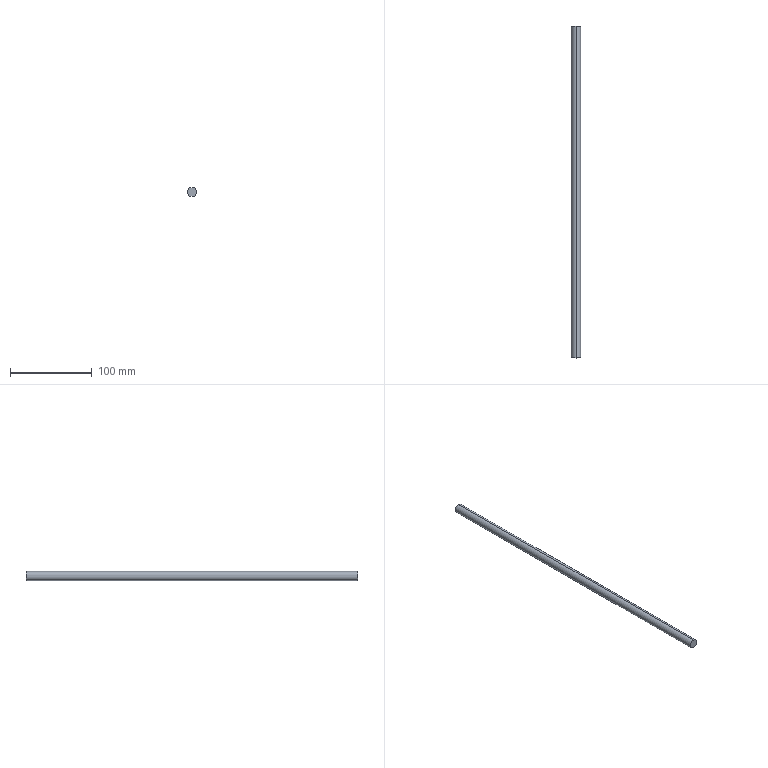Part | STEP file | 4-20.sldasm-Part-405 | 1 solid | 4 faces | box 11.11 x 405 x 11.11 mm | volume 39262 mm3 | cylinder 2 | plane 2 | commonest cylinder face diameters 11.11 x2
STEP:
#1=CARTESIAN_POINT('',(45.,-405.,179.555));
#2=VERTEX_POINT('',#1);
#3=CARTESIAN_POINT('',(45.,-405.,168.445));
#4=VERTEX_POINT('',#3);
#5=CARTESIAN_POINT('',(45.,-405.,174.));
#6=DIRECTION('',(0.,1.,0.));
#7=DIRECTION('',(0.,0.,1.));
#8=AXIS2_PLACEMENT_3D('',#5,#6,#7);
#9=CIRCLE('',#8,5.555);
#10=EDGE_CURVE('',#2,#4,#9,.T.);
#11=ORIENTED_EDGE('',*,*,#10,.T.);
#12=CARTESIAN_POINT('',(45.,0.,168.445));
#13=VERTEX_POINT('',#12);
#14=CARTESIAN_POINT('',(45.,-430.,168.445));
#15=DIRECTION('',(0.,1.,0.));
#16=VECTOR('',#15,1000.);
#17=LINE('',#14,#16);
#18=EDGE_CURVE('',#4,#13,#17,.T.);
#19=ORIENTED_EDGE('',*,*,#18,.T.);
#20=CARTESIAN_POINT('',(45.,0.,179.555));
#21=VERTEX_POINT('',#20);
#22=CARTESIAN_POINT('',(45.,0.,174.));
#23=DIRECTION('',(0.,-1.,0.));
#24=DIRECTION('',(0.,0.,-1.));
#25=AXIS2_PLACEMENT_3D('',#22,#23,#24);
#26=CIRCLE('',#25,5.555);
#27=EDGE_CURVE('',#13,#21,#26,.T.);
#28=ORIENTED_EDGE('',*,*,#27,.T.);
#29=CARTESIAN_POINT('',(45.,-430.,179.555));
#30=DIRECTION('',(0.,1.,0.));
#31=VECTOR('',#30,1000.);
#32=LINE('',#29,#31);
#33=EDGE_CURVE('',#2,#21,#32,.T.);
#34=ORIENTED_EDGE('',*,*,#33,.F.);
#35=EDGE_LOOP('',(#11,#19,#28,#34));
#36=FACE_OUTER_BOUND('',#35,.T.);
#37=CARTESIAN_POINT('',(45.,-430.,174.));
#38=DIRECTION('',(0.,1.,0.));
#39=DIRECTION('',(0.,0.,1.));
#40=AXIS2_PLACEMENT_3D('',#37,#38,#39);
#41=CYLINDRICAL_SURFACE('',#40,5.555);
#42=ADVANCED_FACE('',(#36),#41,.T.);
#43=CARTESIAN_POINT('',(45.,0.,174.));
#44=DIRECTION('',(0.,-1.,0.));
#45=DIRECTION('',(0.,0.,-1.));
#46=AXIS2_PLACEMENT_3D('',#43,#44,#45);
#47=CIRCLE('',#46,5.555);
#48=EDGE_CURVE('',#21,#13,#47,.T.);
#49=ORIENTED_EDGE('',*,*,#48,.F.);
#50=ORIENTED_EDGE('',*,*,#27,.F.);
#51=EDGE_LOOP('',(#49,#50));
#52=FACE_OUTER_BOUND('',#51,.T.);
#53=CARTESIAN_POINT('',(45.,0.,174.));
#54=DIRECTION('',(0.,-1.,0.));
#55=DIRECTION('',(0.,0.,-1.));
#56=AXIS2_PLACEMENT_3D('',#53,#54,#55);
#57=PLANE('',#56);
#58=ADVANCED_FACE('',(#52),#57,.F.);
#59=ORIENTED_EDGE('',*,*,#18,.F.);
#60=CARTESIAN_POINT('',(45.,-405.,174.));
#61=DIRECTION('',(0.,1.,0.));
#62=DIRECTION('',(0.,0.,1.));
#63=AXIS2_PLACEMENT_3D('',#60,#61,#62);
#64=CIRCLE('',#63,5.555);
#65=EDGE_CURVE('',#4,#2,#64,.T.);
#66=ORIENTED_EDGE('',*,*,#65,.T.);
#67=ORIENTED_EDGE('',*,*,#33,.T.);
#68=ORIENTED_EDGE('',*,*,#48,.T.);
#69=EDGE_LOOP('',(#59,#66,#67,#68));
#70=FACE_OUTER_BOUND('',#69,.T.);
#71=CARTESIAN_POINT('',(45.,-430.,174.));
#72=DIRECTION('',(0.,1.,0.));
#73=DIRECTION('',(0.,0.,1.));
#74=AXIS2_PLACEMENT_3D('',#71,#72,#73);
#75=CYLINDRICAL_SURFACE('',#74,5.555);
#76=ADVANCED_FACE('',(#70),#75,.T.);
#77=ORIENTED_EDGE('',*,*,#10,.F.);
#78=ORIENTED_EDGE('',*,*,#65,.F.);
#79=EDGE_LOOP('',(#77,#78));
#80=FACE_OUTER_BOUND('',#79,.T.);
#81=CARTESIAN_POINT('',(120.,-405.,174.));
#82=DIRECTION('',(0.,1.,0.));
#83=DIRECTION('',(0.,0.,1.));
#84=AXIS2_PLACEMENT_3D('',#81,#82,#83);
#85=PLANE('',#84);
#86=ADVANCED_FACE('',(#80),#85,.F.);
#87=CLOSED_SHELL('',(#42,#58,#76,#86));
#88=MANIFOLD_SOLID_BREP('',#87);
#89=CARTESIAN_POINT('',(0.,0.,0.));
#90=DIRECTION('',(0.,0.,1.));
#91=DIRECTION('',(1.,0.,0.));
#92=AXIS2_PLACEMENT_3D('',#89,#90,#91);
#93=(LENGTH_UNIT()NAMED_UNIT(*)SI_UNIT(.MILLI.,.METRE.));
#94=UNCERTAINTY_MEASURE_WITH_UNIT(LENGTH_MEASURE(0.00001),#93,'','');
#95=(NAMED_UNIT(*)PLANE_ANGLE_UNIT()SI_UNIT($,.RADIAN.));
#96=(NAMED_UNIT(*)SI_UNIT($,.STERADIAN.)SOLID_ANGLE_UNIT());
#97=(GEOMETRIC_REPRESENTATION_CONTEXT(3)GLOBAL_UNCERTAINTY_ASSIGNED_CONTEXT((#94))GLOBAL_UNIT_ASSIGNED_CONTEXT((#93,#95,#96))REPRESENTATION_CONTEXT('',''));
#98=ADVANCED_BREP_SHAPE_REPRESENTATION('',(#88,#92),#97);